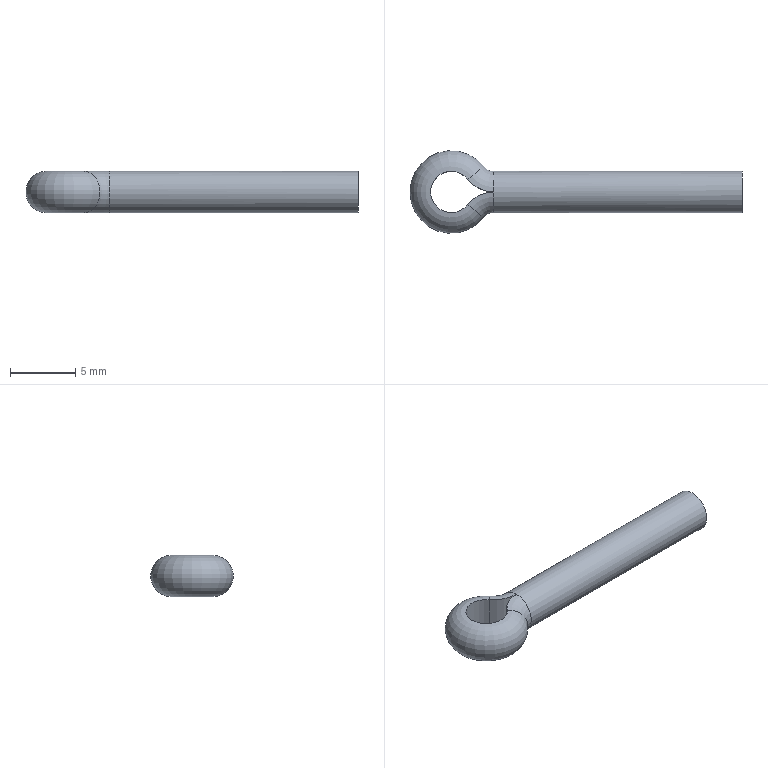Part | NX | features solid 2 | 1 solid | 8 faces | box 25.478 x 6.35 x 3.175 mm | volume 208.616 mm3 | cylinder 4 | torus 3 | plane 1 | commonest cylinder face diameters 3.175 x2 5.08 x2
STEP:
#1=CARTESIAN_POINT('',(-21.052,-0.9769,-1.587));
#2=VERTEX_POINT('',#1);
#3=CARTESIAN_POINT('',(-21.052,-0.9769,1.587));
#4=VERTEX_POINT('',#3);
#5=CARTESIAN_POINT('',(-21.052,-0.9769,-1.587));
#6=DIRECTION('',(0.,0.,1.));
#7=VECTOR('',#6,1000.);
#8=LINE('',#5,#7);
#9=EDGE_CURVE('',#2,#4,#8,.T.);
#10=ORIENTED_EDGE('',*,*,#9,.F.);
#11=CARTESIAN_POINT('',(-21.052,0.9769,-1.587));
#12=VERTEX_POINT('',#11);
#13=CARTESIAN_POINT('',(-22.303,0.,-1.587));
#14=DIRECTION('',(0.,0.,-1.));
#15=DIRECTION('',(-1.,0.,0.));
#16=AXIS2_PLACEMENT_3D('',#13,#14,#15);
#17=CIRCLE('',#16,1.587);
#18=EDGE_CURVE('',#2,#12,#17,.T.);
#19=ORIENTED_EDGE('',*,*,#18,.T.);
#20=CARTESIAN_POINT('',(-21.052,0.9769,1.587));
#21=VERTEX_POINT('',#20);
#22=CARTESIAN_POINT('',(-21.052,0.9769,-1.587));
#23=DIRECTION('',(0.,0.,1.));
#24=VECTOR('',#23,1000.);
#25=LINE('',#22,#24);
#26=EDGE_CURVE('',#12,#21,#25,.T.);
#27=ORIENTED_EDGE('',*,*,#26,.T.);
#28=CARTESIAN_POINT('',(-22.303,0.,1.587));
#29=DIRECTION('',(0.,0.,-1.));
#30=DIRECTION('',(-1.,0.,0.));
#31=AXIS2_PLACEMENT_3D('',#28,#29,#30);
#32=CIRCLE('',#31,1.587);
#33=EDGE_CURVE('',#21,#4,#32,.F.);
#34=ORIENTED_EDGE('',*,*,#33,.T.);
#35=EDGE_LOOP('',(#10,#19,#27,#34));
#36=FACE_BOUND('',#35,.T.);
#37=CARTESIAN_POINT('',(-22.303,0.,0.));
#38=DIRECTION('',(0.,0.,-1.));
#39=DIRECTION('',(-1.,0.,0.));
#40=AXIS2_PLACEMENT_3D('',#37,#38,#39);
#41=CYLINDRICAL_SURFACE('',#40,1.587);
#42=ADVANCED_FACE('',(#36),#41,.F.);
#43=CARTESIAN_POINT('',(-21.052,-0.9769,0.));
#44=DIRECTION('',(0.6154,0.7882,0.));
#45=DIRECTION('',(-0.7882,0.6154,0.));
#46=AXIS2_PLACEMENT_3D('',#43,#44,#45);
#47=CIRCLE('',#46,1.587);
#48=EDGE_CURVE('',#4,#2,#47,.T.);
#49=ORIENTED_EDGE('',*,*,#48,.F.);
#50=ORIENTED_EDGE('',*,*,#33,.F.);
#51=CARTESIAN_POINT('',(-21.052,0.9769,0.));
#52=DIRECTION('',(-0.6154,0.7882,0.));
#53=DIRECTION('',(-0.7882,-0.6154,0.));
#54=AXIS2_PLACEMENT_3D('',#51,#52,#53);
#55=CIRCLE('',#54,1.587);
#56=EDGE_CURVE('',#21,#12,#55,.T.);
#57=ORIENTED_EDGE('',*,*,#56,.T.);
#58=ORIENTED_EDGE('',*,*,#18,.F.);
#59=EDGE_LOOP('',(#49,#50,#57,#58));
#60=FACE_BOUND('',#59,.T.);
#61=CARTESIAN_POINT('',(-22.303,0.,0.));
#62=DIRECTION('',(0.,0.,-1.));
#63=DIRECTION('',(-1.,0.,0.));
#64=AXIS2_PLACEMENT_3D('',#61,#62,#63);
#65=TOROIDAL_SURFACE('',#64,1.587,1.587);
#66=ADVANCED_FACE('',(#60),#65,.T.);
#67=CARTESIAN_POINT('',(-19.05,0.,-1.587));
#68=VERTEX_POINT('',#67);
#69=CARTESIAN_POINT('',(-19.05,0.,1.587));
#70=VERTEX_POINT('',#69);
#71=CARTESIAN_POINT('',(-19.05,0.,-1.587));
#72=DIRECTION('',(0.,0.,1.));
#73=VECTOR('',#72,1000.);
#74=LINE('',#71,#73);
#75=EDGE_CURVE('',#68,#70,#74,.T.);
#76=ORIENTED_EDGE('',*,*,#75,.F.);
#77=CARTESIAN_POINT('',(-19.05,-2.54,-1.587));
#78=DIRECTION('',(0.,0.,1.));
#79=DIRECTION('',(1.,0.,0.));
#80=AXIS2_PLACEMENT_3D('',#77,#78,#79);
#81=CIRCLE('',#80,2.54);
#82=EDGE_CURVE('',#68,#2,#81,.T.);
#83=ORIENTED_EDGE('',*,*,#82,.T.);
#84=ORIENTED_EDGE('',*,*,#9,.T.);
#85=CARTESIAN_POINT('',(-19.05,-2.54,1.587));
#86=DIRECTION('',(0.,0.,1.));
#87=DIRECTION('',(1.,0.,0.));
#88=AXIS2_PLACEMENT_3D('',#85,#86,#87);
#89=CIRCLE('',#88,2.54);
#90=EDGE_CURVE('',#4,#70,#89,.F.);
#91=ORIENTED_EDGE('',*,*,#90,.T.);
#92=EDGE_LOOP('',(#76,#83,#84,#91));
#93=FACE_BOUND('',#92,.T.);
#94=CARTESIAN_POINT('',(-19.05,-2.54,0.));
#95=DIRECTION('',(0.,0.,1.));
#96=DIRECTION('',(1.,0.,0.));
#97=AXIS2_PLACEMENT_3D('',#94,#95,#96);
#98=CYLINDRICAL_SURFACE('',#97,2.54);
#99=ADVANCED_FACE('',(#93),#98,.T.);
#100=CARTESIAN_POINT('',(-19.05,0.,0.));
#101=DIRECTION('',(1.,0.,0.));
#102=DIRECTION('',(0.,1.,0.));
#103=AXIS2_PLACEMENT_3D('',#100,#101,#102);
#104=CIRCLE('',#103,1.587);
#105=EDGE_CURVE('',#70,#68,#104,.T.);
#106=ORIENTED_EDGE('',*,*,#105,.F.);
#107=ORIENTED_EDGE('',*,*,#90,.F.);
#108=ORIENTED_EDGE('',*,*,#48,.T.);
#109=ORIENTED_EDGE('',*,*,#82,.F.);
#110=EDGE_LOOP('',(#106,#107,#108,#109));
#111=FACE_BOUND('',#110,.T.);
#112=CARTESIAN_POINT('',(-19.05,-2.54,0.));
#113=DIRECTION('',(0.,0.,1.));
#114=DIRECTION('',(1.,0.,0.));
#115=AXIS2_PLACEMENT_3D('',#112,#113,#114);
#116=TOROIDAL_SURFACE('',#115,2.54,1.587);
#117=ADVANCED_FACE('',(#111),#116,.T.);
#118=CARTESIAN_POINT('',(0.,1.587,0.));
#119=VERTEX_POINT('',#118);
#120=CARTESIAN_POINT('',(0.,0.,0.));
#121=DIRECTION('',(1.,0.,0.));
#122=DIRECTION('',(0.,1.,0.));
#123=AXIS2_PLACEMENT_3D('',#120,#121,#122);
#124=CIRCLE('',#123,1.587);
#125=EDGE_CURVE('',#119,#119,#124,.T.);
#126=ORIENTED_EDGE('',*,*,#125,.F.);
#127=EDGE_LOOP('',(#126));
#128=FACE_BOUND('',#127,.T.);
#129=CARTESIAN_POINT('',(-19.05,0.,0.));
#130=DIRECTION('',(-1.,0.,0.));
#131=DIRECTION('',(0.,-1.,0.));
#132=AXIS2_PLACEMENT_3D('',#129,#130,#131);
#133=CIRCLE('',#132,1.587);
#134=EDGE_CURVE('',#68,#70,#133,.F.);
#135=ORIENTED_EDGE('',*,*,#134,.T.);
#136=ORIENTED_EDGE('',*,*,#105,.T.);
#137=EDGE_LOOP('',(#135,#136));
#138=FACE_BOUND('',#137,.T.);
#139=CARTESIAN_POINT('',(-19.05,0.,0.));
#140=DIRECTION('',(1.,0.,0.));
#141=DIRECTION('',(0.,0.,-1.));
#142=AXIS2_PLACEMENT_3D('',#139,#140,#141);
#143=CYLINDRICAL_SURFACE('',#142,1.587);
#144=ADVANCED_FACE('',(#128,#138),#143,.T.);
#145=ORIENTED_EDGE('',*,*,#125,.T.);
#146=EDGE_LOOP('',(#145));
#147=FACE_BOUND('',#146,.T.);
#148=CARTESIAN_POINT('',(0.,0.,0.));
#149=DIRECTION('',(1.,0.,0.));
#150=DIRECTION('',(0.,0.,-1.));
#151=AXIS2_PLACEMENT_3D('',#148,#149,#150);
#152=PLANE('',#151);
#153=ADVANCED_FACE('',(#147),#152,.T.);
#154=ORIENTED_EDGE('',*,*,#75,.T.);
#155=CARTESIAN_POINT('',(-19.05,2.54,1.587));
#156=DIRECTION('',(0.,0.,-1.));
#157=DIRECTION('',(1.,0.,0.));
#158=AXIS2_PLACEMENT_3D('',#155,#156,#157);
#159=CIRCLE('',#158,2.54);
#160=EDGE_CURVE('',#21,#70,#159,.F.);
#161=ORIENTED_EDGE('',*,*,#160,.F.);
#162=ORIENTED_EDGE('',*,*,#26,.F.);
#163=CARTESIAN_POINT('',(-19.05,2.54,-1.587));
#164=DIRECTION('',(0.,0.,-1.));
#165=DIRECTION('',(1.,0.,0.));
#166=AXIS2_PLACEMENT_3D('',#163,#164,#165);
#167=CIRCLE('',#166,2.54);
#168=EDGE_CURVE('',#68,#12,#167,.T.);
#169=ORIENTED_EDGE('',*,*,#168,.F.);
#170=EDGE_LOOP('',(#154,#161,#162,#169));
#171=FACE_BOUND('',#170,.T.);
#172=CARTESIAN_POINT('',(-19.05,2.54,0.));
#173=DIRECTION('',(0.,0.,1.));
#174=DIRECTION('',(1.,0.,0.));
#175=AXIS2_PLACEMENT_3D('',#172,#173,#174);
#176=CYLINDRICAL_SURFACE('',#175,2.54);
#177=ADVANCED_FACE('',(#171),#176,.T.);
#178=ORIENTED_EDGE('',*,*,#134,.F.);
#179=ORIENTED_EDGE('',*,*,#168,.T.);
#180=ORIENTED_EDGE('',*,*,#56,.F.);
#181=ORIENTED_EDGE('',*,*,#160,.T.);
#182=EDGE_LOOP('',(#178,#179,#180,#181));
#183=FACE_BOUND('',#182,.T.);
#184=CARTESIAN_POINT('',(-19.05,2.54,0.));
#185=DIRECTION('',(0.,0.,1.));
#186=DIRECTION('',(1.,0.,0.));
#187=AXIS2_PLACEMENT_3D('',#184,#185,#186);
#188=TOROIDAL_SURFACE('',#187,2.54,1.587);
#189=ADVANCED_FACE('',(#183),#188,.T.);
#190=CLOSED_SHELL('',(#42,#66,#99,#117,#144,#153,#177,#189));
#191=MANIFOLD_SOLID_BREP('',#190);
#192=(LENGTH_UNIT()NAMED_UNIT(*)SI_UNIT(.MILLI.,.METRE.));
#193=UNCERTAINTY_MEASURE_WITH_UNIT(LENGTH_MEASURE(0.00001),#192,'','');
#194=(NAMED_UNIT(*)PLANE_ANGLE_UNIT()SI_UNIT($,.RADIAN.));
#195=(NAMED_UNIT(*)SI_UNIT($,.STERADIAN.)SOLID_ANGLE_UNIT());
#196=(GEOMETRIC_REPRESENTATION_CONTEXT(3)GLOBAL_UNCERTAINTY_ASSIGNED_CONTEXT((#193))GLOBAL_UNIT_ASSIGNED_CONTEXT((#192,#194,#195))REPRESENTATION_CONTEXT('',''));
#197=ADVANCED_BREP_SHAPE_REPRESENTATION('',(#191),#196);